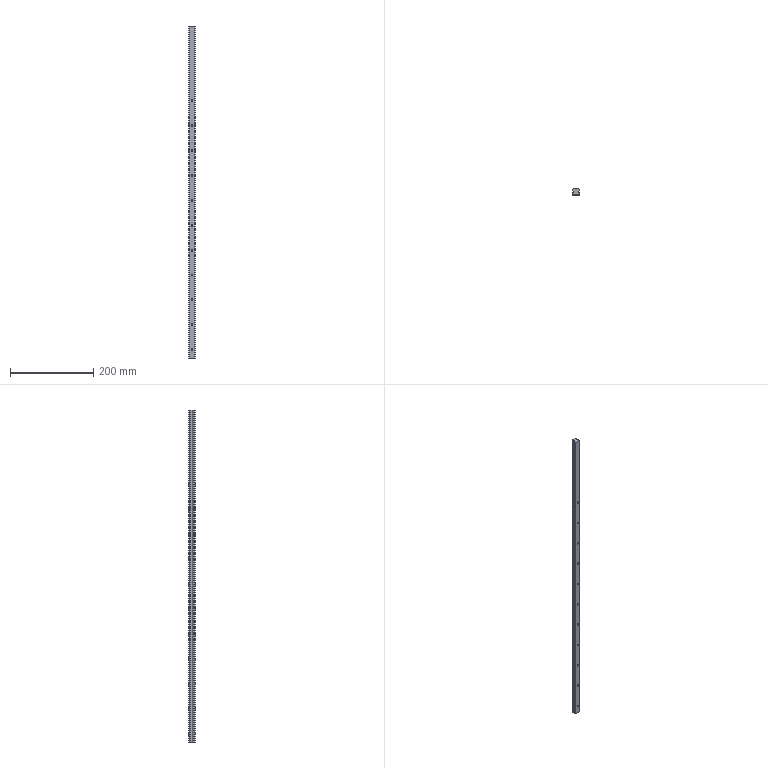Part | STEP file | HGH15 guide rail 3 (HGH15 rail) | 1 solid | 79 faces | box 15 x 15 x 800 mm | volume 153607 mm3 | cylinder 50 | plane 29 | commonest cylinder face diameters 4.5 x22 7.5 x22 0.8 x6